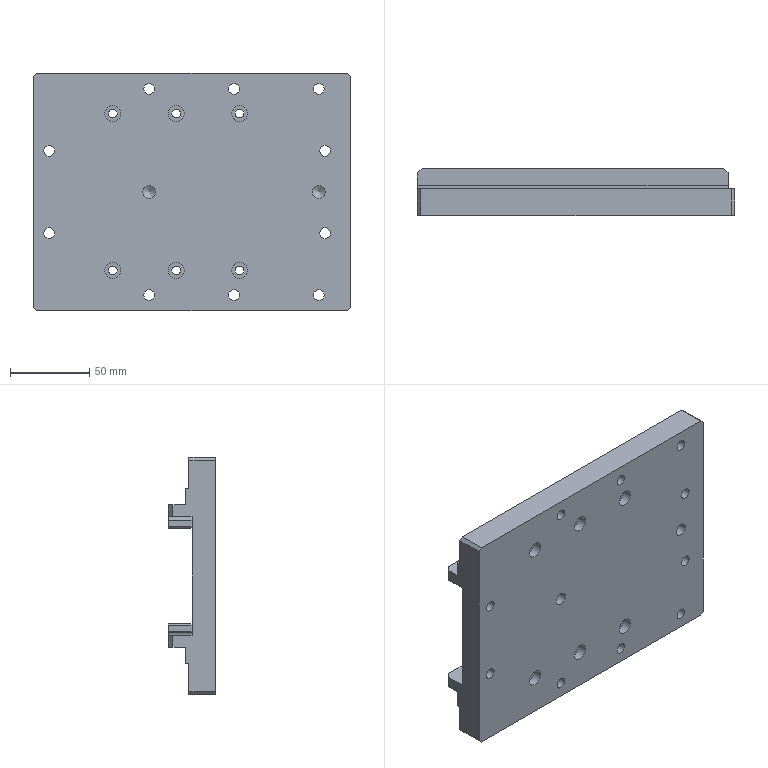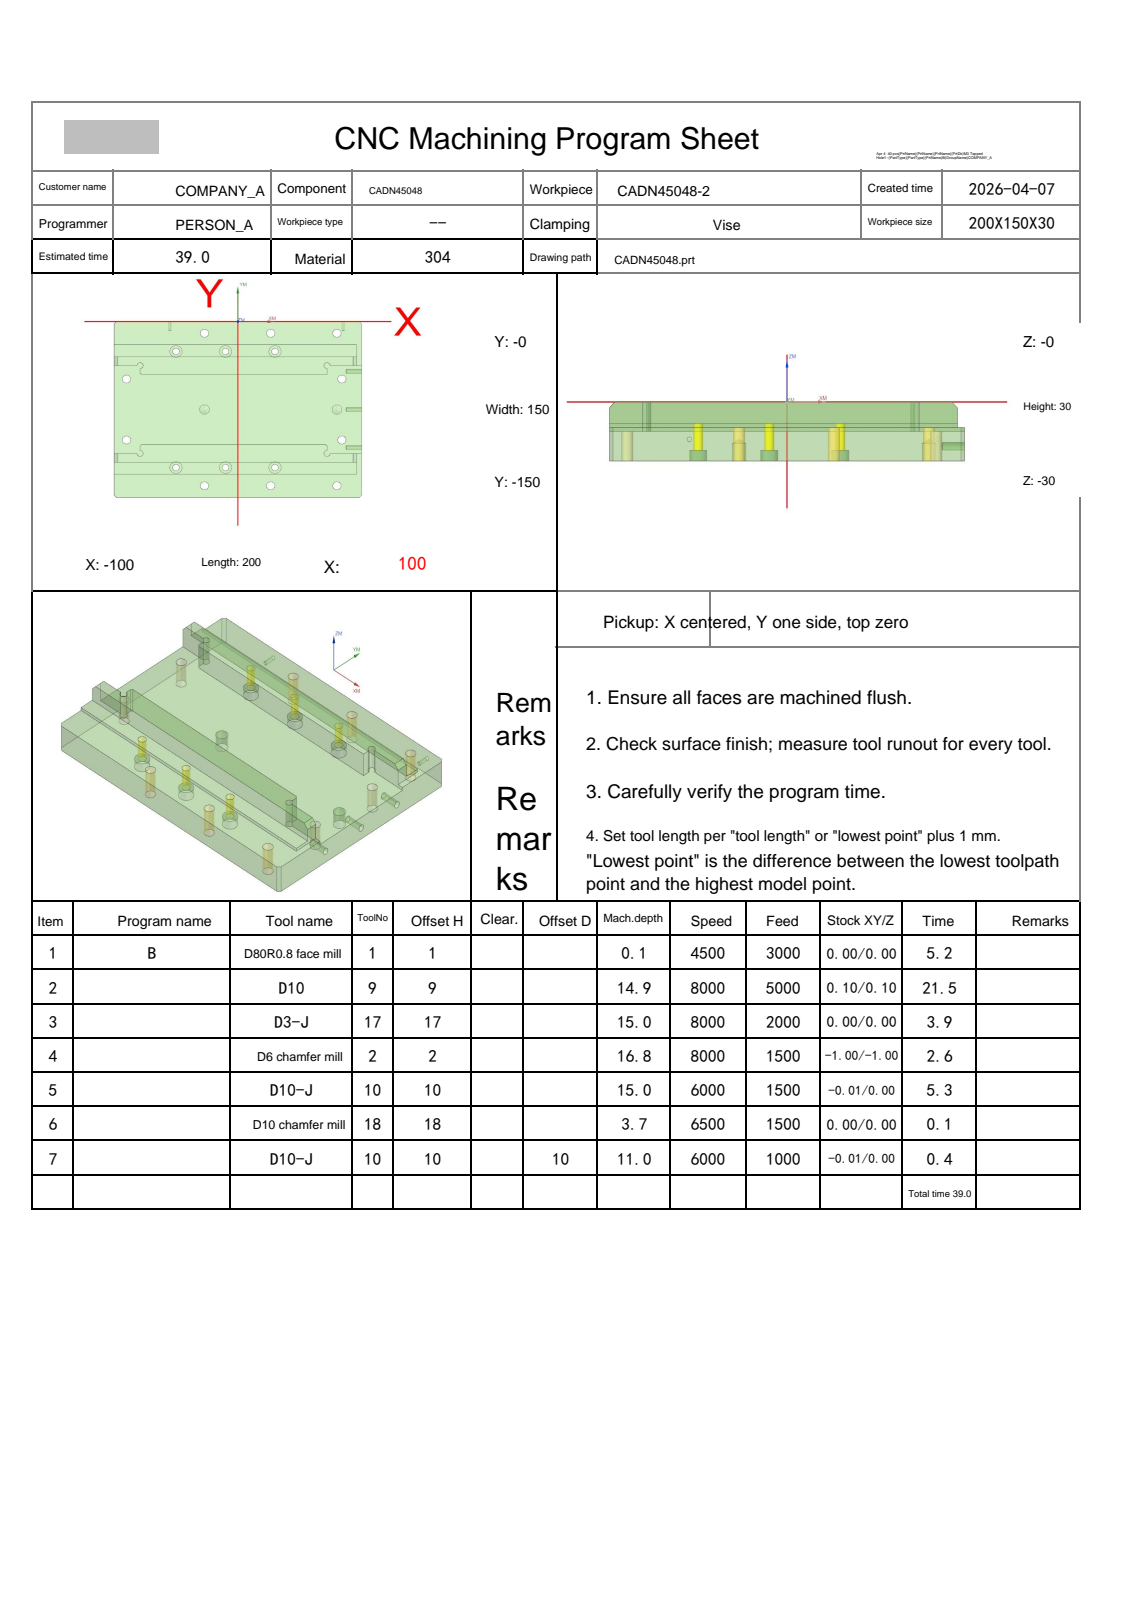NC program | NX | posted by the shop | part box 200 x 30 x 150 mm
Lines 1 to 219 of 19220:
%
O0001
(Machine time: 40.30 MIN)
(===Total Tool:6===)
(T1=D80R0.8 face mill D=80.  R=0.8  D-  H01 Z=0.    )
(T9=D10     D=10.  R=0.   D-  H09 Z=-14.9 )
(T17=D3-J   D=3.   R=0.   D-  H17 Z=-15.  )
(T2=D6 chamfer mill   D=6.   R=0.   D-  H02 Z=-16.8 )
(T10=D10-J  D=10.  R=0.   D10 H10 Z=-15.  )
(T18=D10 chamfer mill D=10.  R=0.   D-  H18 Z=-3.7  )
G80 G90 G17 G49 G40
G91 G28 Z0
M01
N1 T01 M06
(D80R0.8 face mill  D=80. R=0.8 H=01 ce=0.20 di=0.10)
G00 G90 G54 X152. Y-144. M03 S4500
G43 H01 Z20.
M08
Z6.011
G01 Z4.011 F3000.
X140.
X-132.
G02 X-140. Y-136. I0.0 J8.
G01 Y-105.2
G02 X-132.8 Y-98. I7.2 J0.0
G01 X132.8
G03 X140. Y-90.8 I0.0 J7.2
G01 Y-60.
G03 X132. Y-52. I-8. J0.0
G01 X-132.
G02 X-140. Y-44. I0.0 J8.
G01 Y-13.2
G02 X-132.8 Y-6. I7.2 J0.0
G01 X140.
X152.
Z6.011
G00 Z7.5
Y-144.
Z5.522
G01 Z3.522
X140.
X-132.
G02 X-140. Y-136. I0.0 J8.
G01 Y-105.2
G02 X-132.8 Y-98. I7.2 J0.0
G01 X132.8
G03 X140. Y-90.8 I0.0 J7.2
G01 Y-60.
G03 X132. Y-52. I-8. J0.0
G01 X-132.
G02 X-140. Y-44. I0.0 J8.
G01 Y-13.2
G02 X-132.8 Y-6. I7.2 J0.0
G01 X140.
X152.
Z5.522
G00 Z7.011
Y-144.
Z5.033
G01 Z3.033
X140.
X-132.
G02 X-140. Y-136. I0.0 J8.
G01 Y-105.2
G02 X-132.8 Y-98. I7.2 J0.0
G01 X132.8
G03 X140. Y-90.8 I0.0 J7.2
G01 Y-60.
G03 X132. Y-52. I-8. J0.0
G01 X-132.
G02 X-140. Y-44. I0.0 J8.
G01 Y-13.2
G02 X-132.8 Y-6. I7.2 J0.0
G01 X140.
X152.
Z5.033
G00 Z6.522
Y-144.
Z4.544
G01 Z2.544
X140.
X-132.
G02 X-140. Y-136. I0.0 J8.
G01 Y-105.2
G02 X-132.8 Y-98. I7.2 J0.0
G01 X132.8
G03 X140. Y-90.8 I0.0 J7.2
G01 Y-60.
G03 X132. Y-52. I-8. J0.0
G01 X-132.
G02 X-140. Y-44. I0.0 J8.
G01 Y-13.2
G02 X-132.8 Y-6. I7.2 J0.0
G01 X140.
X152.
Z4.544
G00 Z6.033
Y-144.
Z4.056
G01 Z2.056
X140.
X-132.
G02 X-140. Y-136. I0.0 J8.
G01 Y-105.2
G02 X-132.8 Y-98. I7.2 J0.0
G01 X132.8
G03 X140. Y-90.8 I0.0 J7.2
G01 Y-60.
G03 X132. Y-52. I-8. J0.0
G01 X-132.
G02 X-140. Y-44. I0.0 J8.
G01 Y-13.2
G02 X-132.8 Y-6. I7.2 J0.0
G01 X140.
X152.
Z4.056
G00 Z5.544
Y-144.
Z3.567
G01 Z1.567
X140.
X-132.
G02 X-140. Y-136. I0.0 J8.
G01 Y-105.2
G02 X-132.8 Y-98. I7.2 J0.0
G01 X132.8
G03 X140. Y-90.8 I0.0 J7.2
G01 Y-60.
G03 X132. Y-52. I-8. J0.0
G01 X-132.
G02 X-140. Y-44. I0.0 J8.
G01 Y-13.2
G02 X-132.8 Y-6. I7.2 J0.0
G01 X140.
X152.
Z3.567
G00 Z5.056
Y-144.
Z3.078
G01 Z1.078
X140.
X-132.
G02 X-140. Y-136. I0.0 J8.
G01 Y-105.2
G02 X-132.8 Y-98. I7.2 J0.0
G01 X132.8
G03 X140. Y-90.8 I0.0 J7.2
G01 Y-60.
G03 X132. Y-52. I-8. J0.0
G01 X-132.
G02 X-140. Y-44. I0.0 J8.
G01 Y-13.2
G02 X-132.8 Y-6. I7.2 J0.0
G01 X140.
X152.
Z3.078
G00 Z4.567
Y-144.
Z2.589
G01 Z.589
X140.
X-132.
G02 X-140. Y-136. I0.0 J8.
G01 Y-105.2
G02 X-132.8 Y-98. I7.2 J0.0
G01 X132.8
G03 X140. Y-90.8 I0.0 J7.2
G01 Y-60.
G03 X132. Y-52. I-8. J0.0
G01 X-132.
G02 X-140. Y-44. I0.0 J8.
G01 Y-13.2
G02 X-132.8 Y-6. I7.2 J0.0
G01 X140.
X152.
Z2.589
G00 Z4.078
Y-144.
Z2.1
G01 Z.1
X140.
X-132.
G02 X-140. Y-136. I0.0 J8.
G01 Y-105.2
G02 X-132.8 Y-98. I7.2 J0.0
G01 X132.8
G03 X140. Y-90.8 I0.0 J7.2
G01 Y-60.
G03 X132. Y-52. I-8. J0.0
G01 X-132.
G02 X-140. Y-44. I0.0 J8.
G01 Y-13.2
G02 X-132.8 Y-6. I7.2 J0.0
G01 X140.
X152.
Z2.1
G00 Z20.
G00 G90 X152. Y-144. M03 S4500
Z20.
Z2.
G01 Z0.0 F1000.
X140.
X-140.
Y-98.
X140.
Y-52.
X-140.
Y-6.
X140.
X152.
Z2.
G00 Z20.
G91 G28 Z0.0
M05
M09
G91 G28 Z0.0
M01